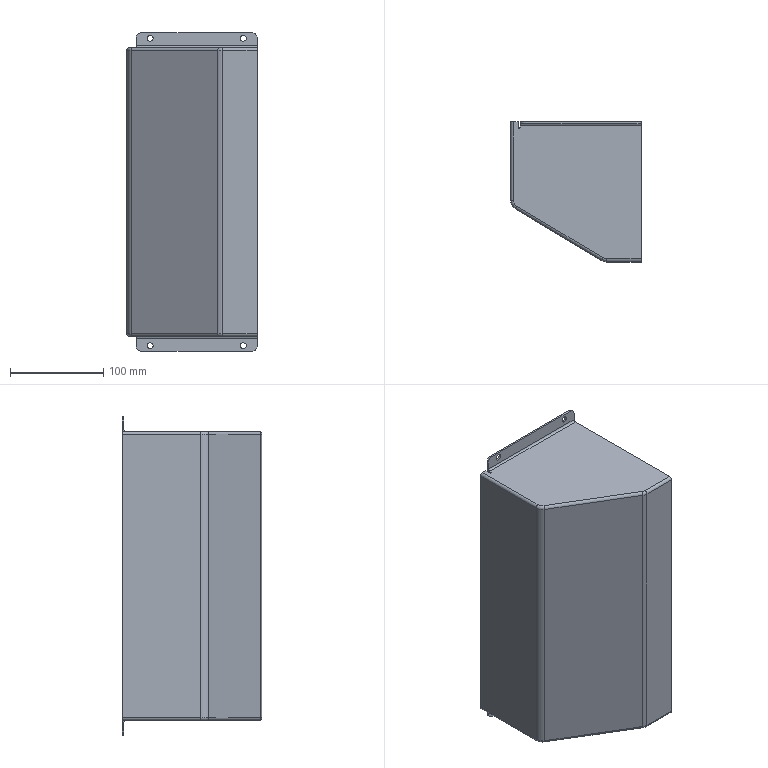Part | STEP file | QA-AD18 | 1 solid | 64 faces | box 140 x 150 x 342 mm | volume 227668 mm3 | cylinder 34 | plane 22 | torus 8 | commonest cylinder face diameters 2 x8 6.5 x8 6 x6 12 x4 4 x2 8 x2